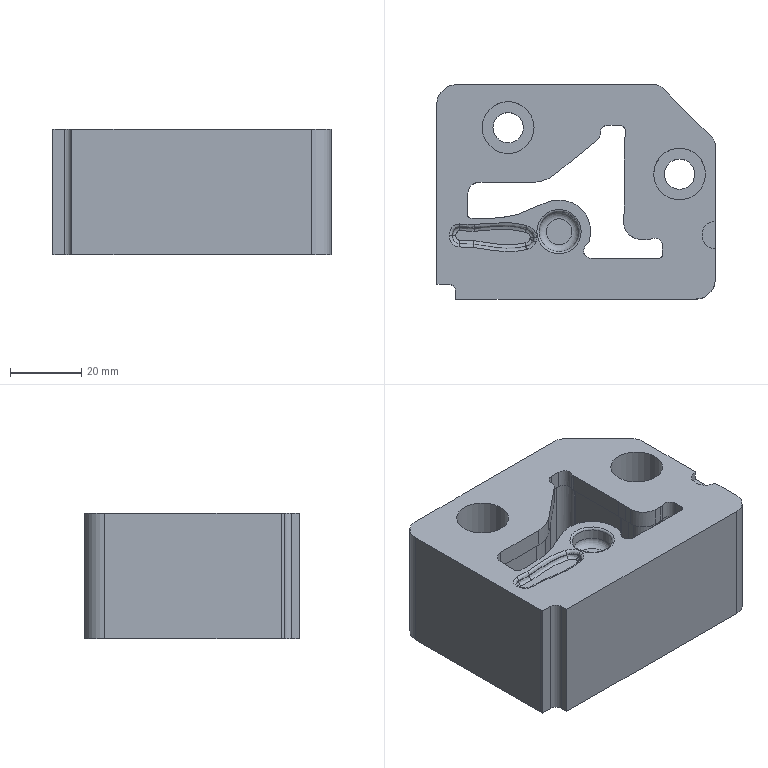Part | NX | features DIE-39 2 | 1 solid | 120 faces | box 78 x 60 x 35 mm | volume 119475 mm3 | spline 66 | plane 38 | cylinder 14 | torus 2 | commonest cylinder face diameters 6 x2 8.506 x2 11 x2 14.5 x2 1.8 x1 2 x1